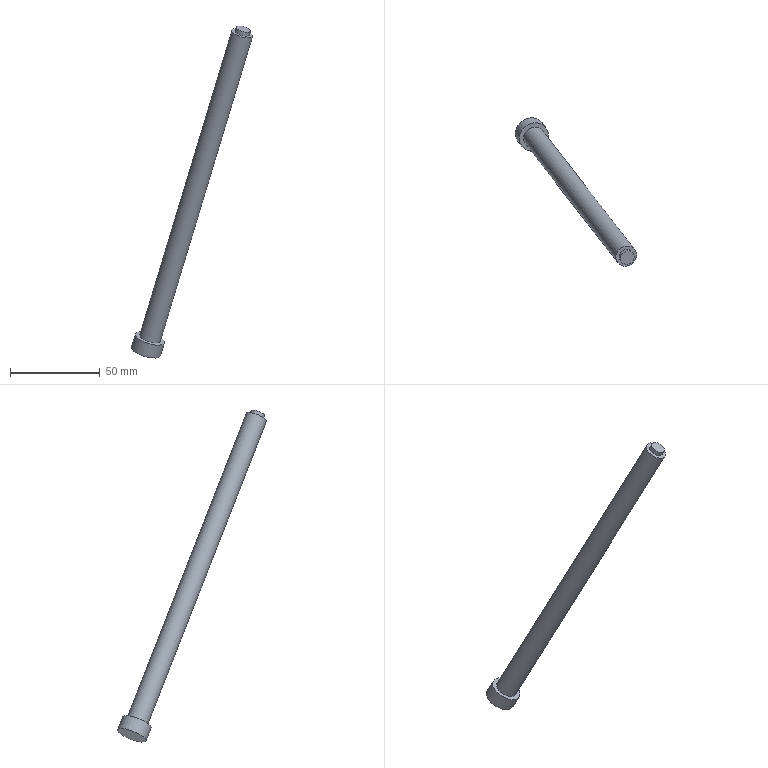Part | STEP file | solid 277 | 1 solid | 7 faces | box 67.648 x 83.054 x 185.27 mm | volume 23432 mm3 | plane 4 | cylinder 3 | commonest cylinder face diameters 8.04 x1 12 x1 17 x1